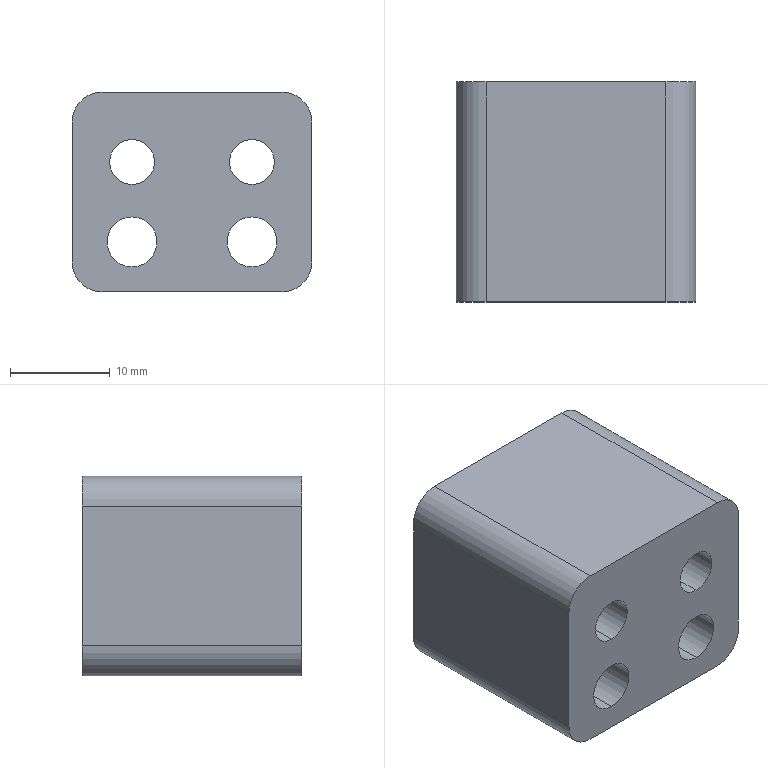Part | STEP file | 1 solid | 24 faces | box 24 x 22 x 20 mm | volume 7795 mm3 | cylinder 16 | plane 8 | commonest cylinder face diameters 4.5 x4 5 x4 6 x4 8 x4